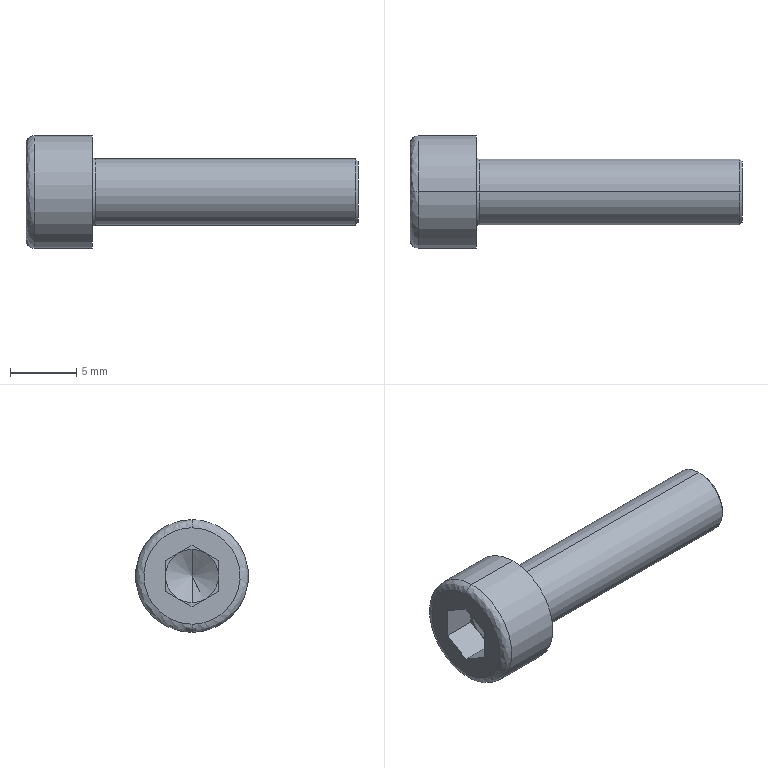Part | SolidWorks | features BaseBody 1 | 1 solid | 27 faces | box 25 x 8.5 x 8.5 mm | volume 634.624 mm3 | plane 15 | spline 4 | cylinder 4 | cone 4 | commonest cylinder face diameters 5 x2 8.5 x2
STEP:
#1=CARTESIAN_POINT('',(5.,0.,2.7));
#2=VERTEX_POINT('',#1);
#3=CARTESIAN_POINT('',(5.,0.,-2.7));
#4=VERTEX_POINT('',#3);
#5=CARTESIAN_POINT('',(5.,0.,2.7));
#6=CARTESIAN_POINT('',(5.,0.1716,2.7));
#7=CARTESIAN_POINT('',(5.,0.4245,2.676));
#8=CARTESIAN_POINT('',(5.,0.7118,2.607));
#9=CARTESIAN_POINT('',(5.,0.8535,2.562));
#10=CARTESIAN_POINT('',(5.,0.9138,2.541));
#11=CARTESIAN_POINT('',(5.,0.9539,2.526));
#12=CARTESIAN_POINT('',(5.,0.9722,2.519));
#13=CARTESIAN_POINT('',(5.,1.34,2.373));
#14=CARTESIAN_POINT('',(5.,1.646,2.172));
#15=CARTESIAN_POINT('',(5.,2.041,1.778));
#16=CARTESIAN_POINT('',(5.,2.215,1.564));
#17=CARTESIAN_POINT('',(5.,2.376,1.288));
#18=CARTESIAN_POINT('',(5.,2.447,1.143));
#19=CARTESIAN_POINT('',(5.,2.475,1.08));
#20=CARTESIAN_POINT('',(5.,2.493,1.037));
#21=CARTESIAN_POINT('',(5.,2.503,1.014));
#22=CARTESIAN_POINT('',(5.,2.637,0.675));
#23=CARTESIAN_POINT('',(5.,2.7,0.343));
#24=CARTESIAN_POINT('',(5.,2.7,-0.1715));
#25=CARTESIAN_POINT('',(5.,2.676,-0.4243));
#26=CARTESIAN_POINT('',(5.,2.607,-0.7117));
#27=CARTESIAN_POINT('',(5.,2.562,-0.8534));
#28=CARTESIAN_POINT('',(5.,2.541,-0.9137));
#29=CARTESIAN_POINT('',(5.,2.526,-0.9539));
#30=CARTESIAN_POINT('',(5.,2.519,-0.9722));
#31=CARTESIAN_POINT('',(5.,2.373,-1.34));
#32=CARTESIAN_POINT('',(5.,2.172,-1.646));
#33=CARTESIAN_POINT('',(5.,1.778,-2.041));
#34=CARTESIAN_POINT('',(5.,1.564,-2.215));
#35=CARTESIAN_POINT('',(5.,1.288,-2.376));
#36=CARTESIAN_POINT('',(5.,1.143,-2.447));
#37=CARTESIAN_POINT('',(5.,1.08,-2.475));
#38=CARTESIAN_POINT('',(5.,1.037,-2.493));
#39=CARTESIAN_POINT('',(5.,1.014,-2.503));
#40=CARTESIAN_POINT('',(5.,0.6748,-2.637));
#41=CARTESIAN_POINT('',(5.,0.3435,-2.7));
#42=CARTESIAN_POINT('',(5.,0.,-2.7));
#43=B_SPLINE_CURVE_WITH_KNOTS('',3,(#5,#6,#7,#8,#9,#10,#11,#12,#13,#14,#15,#16,#17,#18,#19,#20,#21,#22,#23,#24,#25,#26,#27,#28,#29,#30,#31,#32,#33,#34,#35,#36,#37,#38,#39,#40,#41,#42),.UNSPECIFIED.,.F.,.F.,(4,1,1,1,2,2,2,1,1,1,2,2,2,1,1,1,2,2,2,1,1,1,2,2,4),(0.,0.0625,0.09375,0.1094,0.1172,0.125,0.25,0.3125,0.3437,0.3594,0.3672,0.375,0.5,0.5625,0.5937,0.6094,0.6172,0.625,0.75,0.8125,0.8437,0.8594,0.8672,0.875,1.),.UNSPECIFIED.);
#44=EDGE_CURVE('',#2,#4,#43,.T.);
#45=ORIENTED_EDGE('',*,*,#44,.F.);
#46=CARTESIAN_POINT('',(5.2,0.,2.5));
#47=VERTEX_POINT('',#46);
#48=CARTESIAN_POINT('',(5.2,0.,2.7));
#49=DIRECTION('',(0.,-1.,0.));
#50=DIRECTION('',(0.,0.,1.));
#51=AXIS2_PLACEMENT_3D('',#48,#49,#50);
#52=CIRCLE('',#51,0.2);
#53=EDGE_CURVE('',#2,#47,#52,.T.);
#54=ORIENTED_EDGE('',*,*,#53,.T.);
#55=CARTESIAN_POINT('',(5.2,0.,-2.5));
#56=VERTEX_POINT('',#55);
#57=CARTESIAN_POINT('',(5.2,0.,0.));
#58=DIRECTION('',(1.,0.,0.));
#59=DIRECTION('',(0.,0.,1.));
#60=AXIS2_PLACEMENT_3D('',#57,#58,#59);
#61=CIRCLE('',#60,2.5);
#62=EDGE_CURVE('',#56,#47,#61,.T.);
#63=ORIENTED_EDGE('',*,*,#62,.F.);
#64=CARTESIAN_POINT('',(5.2,0.,-2.7));
#65=DIRECTION('',(0.,1.,0.));
#66=DIRECTION('',(0.,0.,-1.));
#67=AXIS2_PLACEMENT_3D('',#64,#65,#66);
#68=CIRCLE('',#67,0.2);
#69=EDGE_CURVE('',#4,#56,#68,.T.);
#70=ORIENTED_EDGE('',*,*,#69,.F.);
#71=EDGE_LOOP('',(#45,#54,#63,#70));
#72=FACE_OUTER_BOUND('',#71,.T.);
#73=CARTESIAN_POINT('',(5.,0.,-2.7));
#74=CARTESIAN_POINT('',(5.,5.4,-2.7));
#75=CARTESIAN_POINT('',(5.,5.4,2.7));
#76=CARTESIAN_POINT('',(5.,0.,2.7));
#77=CARTESIAN_POINT('',(5.,0.,-2.583));
#78=CARTESIAN_POINT('',(5.,5.166,-2.583));
#79=CARTESIAN_POINT('',(5.,5.166,2.583));
#80=CARTESIAN_POINT('',(5.,0.,2.583));
#81=CARTESIAN_POINT('',(5.083,0.,-2.5));
#82=CARTESIAN_POINT('',(5.083,5.,-2.5));
#83=CARTESIAN_POINT('',(5.083,5.,2.5));
#84=CARTESIAN_POINT('',(5.083,0.,2.5));
#85=CARTESIAN_POINT('',(5.2,0.,-2.5));
#86=CARTESIAN_POINT('',(5.2,5.,-2.5));
#87=CARTESIAN_POINT('',(5.2,5.,2.5));
#88=CARTESIAN_POINT('',(5.2,0.,2.5));
#89=(BOUNDED_SURFACE()B_SPLINE_SURFACE(3,3,((#73,#74,#75,#76),(#77,#78,#79,#80),(#81,#82,#83,#84),(#85,#86,#87,#88)),.UNSPECIFIED.,.F.,.F.,.T.)B_SPLINE_SURFACE_WITH_KNOTS((4,4),(4,4),(0.,1.),(0.,1.),.UNSPECIFIED.)GEOMETRIC_REPRESENTATION_ITEM()RATIONAL_B_SPLINE_SURFACE(((1.,0.3333,0.3333,1.),(0.8047,0.2682,0.2682,0.8047),(0.8047,0.2682,0.2682,0.8047),(1.,0.3333,0.3333,1.)))REPRESENTATION_ITEM('')SURFACE());
#90=ADVANCED_FACE('',(#72),#89,.F.);
#91=CARTESIAN_POINT('',(0.625,0.,4.25));
#92=VERTEX_POINT('',#91);
#93=CARTESIAN_POINT('',(0.625,0.,-4.25));
#94=VERTEX_POINT('',#93);
#95=CARTESIAN_POINT('',(0.625,0.,0.));
#96=DIRECTION('',(1.,0.,0.));
#97=DIRECTION('',(0.,0.,1.));
#98=AXIS2_PLACEMENT_3D('',#95,#96,#97);
#99=CIRCLE('',#98,4.25);
#100=EDGE_CURVE('',#92,#94,#99,.T.);
#101=ORIENTED_EDGE('',*,*,#100,.F.);
#102=CARTESIAN_POINT('',(0.,0.,3.625));
#103=VERTEX_POINT('',#102);
#104=CARTESIAN_POINT('',(0.625,0.,3.625));
#105=DIRECTION('',(0.,-1.,0.));
#106=DIRECTION('',(0.,0.,1.));
#107=AXIS2_PLACEMENT_3D('',#104,#105,#106);
#108=CIRCLE('',#107,0.625);
#109=EDGE_CURVE('',#92,#103,#108,.T.);
#110=ORIENTED_EDGE('',*,*,#109,.T.);
#111=CARTESIAN_POINT('',(0.,0.,-3.625));
#112=VERTEX_POINT('',#111);
#113=CARTESIAN_POINT('',(0.,0.,3.625));
#114=CARTESIAN_POINT('',(0.,-7.25,3.625));
#115=CARTESIAN_POINT('',(0.,-7.25,-3.625));
#116=CARTESIAN_POINT('',(0.,0.,-3.625));
#117=(BOUNDED_CURVE()B_SPLINE_CURVE(3,(#113,#114,#115,#116),.UNSPECIFIED.,.F.,.F.)B_SPLINE_CURVE_WITH_KNOTS((4,4),(0.,1.),.UNSPECIFIED.)CURVE()GEOMETRIC_REPRESENTATION_ITEM()RATIONAL_B_SPLINE_CURVE((1.,0.3333,0.3333,1.))REPRESENTATION_ITEM(''));
#118=EDGE_CURVE('',#103,#112,#117,.T.);
#119=ORIENTED_EDGE('',*,*,#118,.T.);
#120=CARTESIAN_POINT('',(0.625,0.,-3.625));
#121=DIRECTION('',(0.,1.,0.));
#122=DIRECTION('',(0.,0.,-1.));
#123=AXIS2_PLACEMENT_3D('',#120,#121,#122);
#124=CIRCLE('',#123,0.625);
#125=EDGE_CURVE('',#94,#112,#124,.T.);
#126=ORIENTED_EDGE('',*,*,#125,.F.);
#127=EDGE_LOOP('',(#101,#110,#119,#126));
#128=FACE_OUTER_BOUND('',#127,.T.);
#129=CARTESIAN_POINT('',(0.625,0.,4.25));
#130=CARTESIAN_POINT('',(0.625,-8.5,4.25));
#131=CARTESIAN_POINT('',(0.625,-8.5,-4.25));
#132=CARTESIAN_POINT('',(0.625,0.,-4.25));
#133=CARTESIAN_POINT('',(0.2589,0.,4.25));
#134=CARTESIAN_POINT('',(0.2589,-8.5,4.25));
#135=CARTESIAN_POINT('',(0.2589,-8.5,-4.25));
#136=CARTESIAN_POINT('',(0.2589,0.,-4.25));
#137=CARTESIAN_POINT('',(0.,0.,3.991));
#138=CARTESIAN_POINT('',(0.,-7.982,3.991));
#139=CARTESIAN_POINT('',(0.,-7.982,-3.991));
#140=CARTESIAN_POINT('',(0.,0.,-3.991));
#141=CARTESIAN_POINT('',(0.,0.,3.625));
#142=CARTESIAN_POINT('',(0.,-7.25,3.625));
#143=CARTESIAN_POINT('',(0.,-7.25,-3.625));
#144=CARTESIAN_POINT('',(0.,0.,-3.625));
#145=(BOUNDED_SURFACE()B_SPLINE_SURFACE(3,3,((#129,#130,#131,#132),(#133,#134,#135,#136),(#137,#138,#139,#140),(#141,#142,#143,#144)),.UNSPECIFIED.,.F.,.F.,.T.)B_SPLINE_SURFACE_WITH_KNOTS((4,4),(4,4),(0.,1.),(0.,1.),.UNSPECIFIED.)GEOMETRIC_REPRESENTATION_ITEM()RATIONAL_B_SPLINE_SURFACE(((1.,0.3333,0.3333,1.),(0.8047,0.2682,0.2682,0.8047),(0.8047,0.2682,0.2682,0.8047),(1.,0.3333,0.3333,1.)))REPRESENTATION_ITEM('')SURFACE());
#146=ADVANCED_FACE('',(#128),#145,.T.);
#147=CARTESIAN_POINT('',(24.8,0.,2.5));
#148=VERTEX_POINT('',#147);
#149=CARTESIAN_POINT('',(24.8,0.,-2.5));
#150=VERTEX_POINT('',#149);
#151=CARTESIAN_POINT('',(24.8,0.,0.));
#152=DIRECTION('',(-1.,0.,0.));
#153=DIRECTION('',(0.,0.,1.));
#154=AXIS2_PLACEMENT_3D('',#151,#152,#153);
#155=CIRCLE('',#154,2.5);
#156=EDGE_CURVE('',#148,#150,#155,.T.);
#157=ORIENTED_EDGE('',*,*,#156,.T.);
#158=CARTESIAN_POINT('',(25.,0.,-2.5));
#159=DIRECTION('',(-1.,0.,0.));
#160=VECTOR('',#159,1000.);
#161=LINE('',#158,#160);
#162=EDGE_CURVE('',#150,#56,#161,.T.);
#163=ORIENTED_EDGE('',*,*,#162,.T.);
#164=ORIENTED_EDGE('',*,*,#62,.T.);
#165=CARTESIAN_POINT('',(25.,0.,2.5));
#166=DIRECTION('',(-1.,0.,0.));
#167=VECTOR('',#166,1000.);
#168=LINE('',#165,#167);
#169=EDGE_CURVE('',#148,#47,#168,.T.);
#170=ORIENTED_EDGE('',*,*,#169,.F.);
#171=EDGE_LOOP('',(#157,#163,#164,#170));
#172=FACE_OUTER_BOUND('',#171,.T.);
#173=CARTESIAN_POINT('',(25.,0.,0.));
#174=DIRECTION('',(-1.,0.,0.));
#175=DIRECTION('',(0.,0.,1.));
#176=AXIS2_PLACEMENT_3D('',#173,#174,#175);
#177=CYLINDRICAL_SURFACE('',#176,2.5);
#178=ADVANCED_FACE('',(#172),#177,.T.);
#179=CARTESIAN_POINT('',(25.,0.,2.3));
#180=VERTEX_POINT('',#179);
#181=CARTESIAN_POINT('',(25.,0.,-2.3));
#182=VERTEX_POINT('',#181);
#183=CARTESIAN_POINT('',(25.,0.,0.));
#184=DIRECTION('',(-1.,0.,0.));
#185=DIRECTION('',(0.,0.,1.));
#186=AXIS2_PLACEMENT_3D('',#183,#184,#185);
#187=CIRCLE('',#186,2.3);
#188=EDGE_CURVE('',#180,#182,#187,.T.);
#189=ORIENTED_EDGE('',*,*,#188,.T.);
#190=CARTESIAN_POINT('',(24.8,0.,-2.5));
#191=DIRECTION('',(-0.7071,0.,-0.7071));
#192=VECTOR('',#191,1000.);
#193=LINE('',#190,#192);
#194=EDGE_CURVE('',#182,#150,#193,.T.);
#195=ORIENTED_EDGE('',*,*,#194,.T.);
#196=ORIENTED_EDGE('',*,*,#156,.F.);
#197=CARTESIAN_POINT('',(24.8,0.,2.5));
#198=DIRECTION('',(-0.7071,0.,0.7071));
#199=VECTOR('',#198,1000.);
#200=LINE('',#197,#199);
#201=EDGE_CURVE('',#180,#148,#200,.T.);
#202=ORIENTED_EDGE('',*,*,#201,.F.);
#203=EDGE_LOOP('',(#189,#195,#196,#202));
#204=FACE_OUTER_BOUND('',#203,.T.);
#205=CARTESIAN_POINT('',(24.8,0.,0.));
#206=DIRECTION('',(-1.,0.,0.));
#207=DIRECTION('',(0.,0.,1.));
#208=AXIS2_PLACEMENT_3D('',#205,#206,#207);
#209=CONICAL_SURFACE('',#208,2.5,0.7854);
#210=ADVANCED_FACE('',(#204),#209,.T.);
#211=CARTESIAN_POINT('',(5.,0.,-4.25));
#212=VERTEX_POINT('',#211);
#213=CARTESIAN_POINT('',(5.,0.,4.25));
#214=VERTEX_POINT('',#213);
#215=CARTESIAN_POINT('',(5.,0.,0.));
#216=DIRECTION('',(1.,0.,0.));
#217=DIRECTION('',(0.,0.,1.));
#218=AXIS2_PLACEMENT_3D('',#215,#216,#217);
#219=CIRCLE('',#218,4.25);
#220=EDGE_CURVE('',#212,#214,#219,.T.);
#221=ORIENTED_EDGE('',*,*,#220,.F.);
#222=CARTESIAN_POINT('',(5.,0.,-4.25));
#223=DIRECTION('',(-1.,0.,0.));
#224=VECTOR('',#223,1000.);
#225=LINE('',#222,#224);
#226=EDGE_CURVE('',#212,#94,#225,.T.);
#227=ORIENTED_EDGE('',*,*,#226,.T.);
#228=CARTESIAN_POINT('',(0.625,0.,0.));
#229=DIRECTION('',(1.,0.,0.));
#230=DIRECTION('',(0.,0.,1.));
#231=AXIS2_PLACEMENT_3D('',#228,#229,#230);
#232=CIRCLE('',#231,4.25);
#233=EDGE_CURVE('',#94,#92,#232,.T.);
#234=ORIENTED_EDGE('',*,*,#233,.T.);
#235=CARTESIAN_POINT('',(5.,0.,4.25));
#236=DIRECTION('',(-1.,0.,0.));
#237=VECTOR('',#236,1000.);
#238=LINE('',#235,#237);
#239=EDGE_CURVE('',#214,#92,#238,.T.);
#240=ORIENTED_EDGE('',*,*,#239,.F.);
#241=EDGE_LOOP('',(#221,#227,#234,#240));
#242=FACE_OUTER_BOUND('',#241,.T.);
#243=CARTESIAN_POINT('',(5.,0.,0.));
#244=DIRECTION('',(-1.,0.,0.));
#245=DIRECTION('',(0.,0.,1.));
#246=AXIS2_PLACEMENT_3D('',#243,#244,#245);
#247=CYLINDRICAL_SURFACE('',#246,4.25);
#248=ADVANCED_FACE('',(#242),#247,.T.);
#249=CARTESIAN_POINT('',(3.655,0.,0.));
#250=VERTEX_POINT('',#249);
#251=CARTESIAN_POINT('',(2.5,0.,2.));
#252=VERTEX_POINT('',#251);
#253=CARTESIAN_POINT('',(2.5,0.,2.));
#254=DIRECTION('',(-0.5,0.,0.866));
#255=VECTOR('',#254,1000.);
#256=LINE('',#253,#255);
#257=EDGE_CURVE('',#250,#252,#256,.T.);
#258=ORIENTED_EDGE('',*,*,#257,.F.);
#259=CARTESIAN_POINT('',(2.5,0.,-2.));
#260=VERTEX_POINT('',#259);
#261=CARTESIAN_POINT('',(2.5,0.,-2.));
#262=DIRECTION('',(-0.5,0.,-0.866));
#263=VECTOR('',#262,1000.);
#264=LINE('',#261,#263);
#265=EDGE_CURVE('',#250,#260,#264,.T.);
#266=ORIENTED_EDGE('',*,*,#265,.T.);
#267=CARTESIAN_POINT('',(2.5,-1.,-1.732));
#268=VERTEX_POINT('',#267);
#269=CARTESIAN_POINT('',(2.5,0.,0.));
#270=DIRECTION('',(1.,0.,0.));
#271=DIRECTION('',(0.,0.,1.));
#272=AXIS2_PLACEMENT_3D('',#269,#270,#271);
#273=CIRCLE('',#272,2.);
#274=EDGE_CURVE('',#268,#260,#273,.T.);
#275=ORIENTED_EDGE('',*,*,#274,.F.);
#276=CARTESIAN_POINT('',(2.5,-2.,0.));
#277=VERTEX_POINT('',#276);
#278=CARTESIAN_POINT('',(2.5,0.,0.));
#279=DIRECTION('',(-1.,0.,0.));
#280=DIRECTION('',(0.,0.,1.));
#281=AXIS2_PLACEMENT_3D('',#278,#279,#280);
#282=CIRCLE('',#281,2.);
#283=EDGE_CURVE('',#268,#277,#282,.T.);
#284=ORIENTED_EDGE('',*,*,#283,.T.);
#285=CARTESIAN_POINT('',(2.5,-1.,1.732));
#286=VERTEX_POINT('',#285);
#287=CARTESIAN_POINT('',(2.5,0.,0.));
#288=DIRECTION('',(1.,0.,0.));
#289=DIRECTION('',(0.,0.,1.));
#290=AXIS2_PLACEMENT_3D('',#287,#288,#289);
#291=CIRCLE('',#290,2.);
#292=EDGE_CURVE('',#286,#277,#291,.T.);
#293=ORIENTED_EDGE('',*,*,#292,.F.);
#294=CARTESIAN_POINT('',(2.5,0.,0.));
#295=DIRECTION('',(1.,0.,0.));
#296=DIRECTION('',(0.,0.,1.));
#297=AXIS2_PLACEMENT_3D('',#294,#295,#296);
#298=CIRCLE('',#297,2.);
#299=EDGE_CURVE('',#252,#286,#298,.T.);
#300=ORIENTED_EDGE('',*,*,#299,.F.);
#301=EDGE_LOOP('',(#258,#266,#275,#284,#293,#300));
#302=FACE_OUTER_BOUND('',#301,.T.);
#303=CARTESIAN_POINT('',(2.5,0.,0.));
#304=DIRECTION('',(-1.,0.,0.));
#305=DIRECTION('',(0.,0.,1.));
#306=AXIS2_PLACEMENT_3D('',#303,#304,#305);
#307=CONICAL_SURFACE('',#306,2.,1.047);
#308=ADVANCED_FACE('',(#302),#307,.F.);
#309=ORIENTED_EDGE('',*,*,#162,.F.);
#310=CARTESIAN_POINT('',(24.8,0.,0.));
#311=DIRECTION('',(-1.,0.,0.));
#312=DIRECTION('',(0.,0.,1.));
#313=AXIS2_PLACEMENT_3D('',#310,#311,#312);
#314=CIRCLE('',#313,2.5);
#315=EDGE_CURVE('',#150,#148,#314,.T.);
#316=ORIENTED_EDGE('',*,*,#315,.T.);
#317=ORIENTED_EDGE('',*,*,#169,.T.);
#318=CARTESIAN_POINT('',(5.2,0.,0.));
#319=DIRECTION('',(1.,0.,0.));
#320=DIRECTION('',(0.,0.,1.));
#321=AXIS2_PLACEMENT_3D('',#318,#319,#320);
#322=CIRCLE('',#321,2.5);
#323=EDGE_CURVE('',#47,#56,#322,.T.);
#324=ORIENTED_EDGE('',*,*,#323,.T.);
#325=EDGE_LOOP('',(#309,#316,#317,#324));
#326=FACE_OUTER_BOUND('',#325,.T.);
#327=CARTESIAN_POINT('',(25.,0.,0.));
#328=DIRECTION('',(-1.,0.,0.));
#329=DIRECTION('',(0.,0.,1.));
#330=AXIS2_PLACEMENT_3D('',#327,#328,#329);
#331=CYLINDRICAL_SURFACE('',#330,2.5);
#332=ADVANCED_FACE('',(#326),#331,.T.);
#333=ORIENTED_EDGE('',*,*,#53,.F.);
#334=CARTESIAN_POINT('',(5.,0.,-2.7));
#335=CARTESIAN_POINT('',(5.,-0.1716,-2.7));
#336=CARTESIAN_POINT('',(5.,-0.4245,-2.676));
#337=CARTESIAN_POINT('',(5.,-0.7118,-2.607));
#338=CARTESIAN_POINT('',(5.,-0.8535,-2.562));
#339=CARTESIAN_POINT('',(5.,-0.9138,-2.541));
#340=CARTESIAN_POINT('',(5.,-0.9539,-2.526));
#341=CARTESIAN_POINT('',(5.,-0.9722,-2.519));
#342=CARTESIAN_POINT('',(5.,-1.34,-2.373));
#343=CARTESIAN_POINT('',(5.,-1.646,-2.172));
#344=CARTESIAN_POINT('',(5.,-2.041,-1.778));
#345=CARTESIAN_POINT('',(5.,-2.215,-1.564));
#346=CARTESIAN_POINT('',(5.,-2.376,-1.288));
#347=CARTESIAN_POINT('',(5.,-2.447,-1.143));
#348=CARTESIAN_POINT('',(5.,-2.475,-1.08));
#349=CARTESIAN_POINT('',(5.,-2.493,-1.037));
#350=CARTESIAN_POINT('',(5.,-2.503,-1.014));
#351=CARTESIAN_POINT('',(5.,-2.637,-0.675));
#352=CARTESIAN_POINT('',(5.,-2.7,-0.343));
#353=CARTESIAN_POINT('',(5.,-2.7,0.1715));
#354=CARTESIAN_POINT('',(5.,-2.676,0.4243));
#355=CARTESIAN_POINT('',(5.,-2.607,0.7117));
#356=CARTESIAN_POINT('',(5.,-2.562,0.8534));
#357=CARTESIAN_POINT('',(5.,-2.541,0.9137));
#358=CARTESIAN_POINT('',(5.,-2.526,0.9539));
#359=CARTESIAN_POINT('',(5.,-2.519,0.9722));
#360=CARTESIAN_POINT('',(5.,-2.373,1.34));
#361=CARTESIAN_POINT('',(5.,-2.172,1.646));
#362=CARTESIAN_POINT('',(5.,-1.778,2.041));
#363=CARTESIAN_POINT('',(5.,-1.564,2.215));
#364=CARTESIAN_POINT('',(5.,-1.288,2.376));
#365=CARTESIAN_POINT('',(5.,-1.143,2.447));
#366=CARTESIAN_POINT('',(5.,-1.08,2.475));
#367=CARTESIAN_POINT('',(5.,-1.037,2.493));
#368=CARTESIAN_POINT('',(5.,-1.014,2.503));
#369=CARTESIAN_POINT('',(5.,-0.6748,2.637));
#370=CARTESIAN_POINT('',(5.,-0.3435,2.7));
#371=CARTESIAN_POINT('',(5.,0.,2.7));
#372=B_SPLINE_CURVE_WITH_KNOTS('',3,(#334,#335,#336,#337,#338,#339,#340,#341,#342,#343,#344,#345,#346,#347,#348,#349,#350,#351,#352,#353,#354,#355,#356,#357,#358,#359,#360,#361,#362,#363,#364,#365,#366,#367,#368,#369,#370,#371),.UNSPECIFIED.,.F.,.F.,(4,1,1,1,2,2,2,1,1,1,2,2,2,1,1,1,2,2,2,1,1,1,2,2,4),(0.,0.0625,0.09375,0.1094,0.1172,0.125,0.25,0.3125,0.3437,0.3594,0.3672,0.375,0.5,0.5625,0.5937,0.6094,0.6172,0.625,0.75,0.8125,0.8437,0.8594,0.8672,0.875,1.),.UNSPECIFIED.);
#373=EDGE_CURVE('',#4,#2,#372,.T.);
#374=ORIENTED_EDGE('',*,*,#373,.F.);
#375=ORIENTED_EDGE('',*,*,#69,.T.);
#376=ORIENTED_EDGE('',*,*,#323,.F.);
#377=EDGE_LOOP('',(#333,#374,#375,#376));
#378=FACE_OUTER_BOUND('',#377,.T.);
#379=CARTESIAN_POINT('',(5.,0.,2.7));
#380=CARTESIAN_POINT('',(5.,-5.4,2.7));
#381=CARTESIAN_POINT('',(5.,-5.4,-2.7));
#382=CARTESIAN_POINT('',(5.,0.,-2.7));
#383=CARTESIAN_POINT('',(5.,0.,2.583));
#384=CARTESIAN_POINT('',(5.,-5.166,2.583));
#385=CARTESIAN_POINT('',(5.,-5.166,-2.583));
#386=CARTESIAN_POINT('',(5.,0.,-2.583));
#387=CARTESIAN_POINT('',(5.083,0.,2.5));
#388=CARTESIAN_POINT('',(5.083,-5.,2.5));
#389=CARTESIAN_POINT('',(5.083,-5.,-2.5));
#390=CARTESIAN_POINT('',(5.083,0.,-2.5));
#391=CARTESIAN_POINT('',(5.2,0.,2.5));
#392=CARTESIAN_POINT('',(5.2,-5.,2.5));
#393=CARTESIAN_POINT('',(5.2,-5.,-2.5));
#394=CARTESIAN_POINT('',(5.2,0.,-2.5));
#395=(BOUNDED_SURFACE()B_SPLINE_SURFACE(3,3,((#379,#380,#381,#382),(#383,#384,#385,#386),(#387,#388,#389,#390),(#391,#392,#393,#394)),.UNSPECIFIED.,.F.,.F.,.T.)B_SPLINE_SURFACE_WITH_KNOTS((4,4),(4,4),(0.,1.),(0.,1.),.UNSPECIFIED.)GEOMETRIC_REPRESENTATION_ITEM()RATIONAL_B_SPLINE_SURFACE(((1.,0.3333,0.3333,1.),(0.8047,0.2682,0.2682,0.8047),(0.8047,0.2682,0.2682,0.8047),(1.,0.3333,0.3333,1.)))REPRESENTATION_ITEM('')SURFACE());
#396=ADVANCED_FACE('',(#378),#395,.F.);
#397=ORIENTED_EDGE('',*,*,#194,.F.);
#398=CARTESIAN_POINT('',(25.,0.,0.));
#399=DIRECTION('',(-1.,0.,0.));
#400=DIRECTION('',(0.,0.,1.));
#401=AXIS2_PLACEMENT_3D('',#398,#399,#400);
#402=CIRCLE('',#401,2.3);
#403=EDGE_CURVE('',#182,#180,#402,.T.);
#404=ORIENTED_EDGE('',*,*,#403,.T.);
#405=ORIENTED_EDGE('',*,*,#201,.T.);
#406=ORIENTED_EDGE('',*,*,#315,.F.);
#407=EDGE_LOOP('',(#397,#404,#405,#406));
#408=FACE_OUTER_BOUND('',#407,.T.);
#409=CARTESIAN_POINT('',(24.8,0.,0.));
#410=DIRECTION('',(-1.,0.,0.));
#411=DIRECTION('',(0.,0.,1.));
#412=AXIS2_PLACEMENT_3D('',#409,#410,#411);
#413=CONICAL_SURFACE('',#412,2.5,0.7854);
#414=ADVANCED_FACE('',(#408),#413,.T.);
#415=CARTESIAN_POINT('',(5.,0.,0.));
#416=DIRECTION('',(1.,0.,0.));
#417=DIRECTION('',(0.,0.,1.));
#418=AXIS2_PLACEMENT_3D('',#415,#416,#417);
#419=CIRCLE('',#418,4.25);
#420=EDGE_CURVE('',#214,#212,#419,.T.);
#421=ORIENTED_EDGE('',*,*,#420,.T.);
#422=ORIENTED_EDGE('',*,*,#220,.T.);
#423=EDGE_LOOP('',(#421,#422));
#424=FACE_OUTER_BOUND('',#423,.T.);
#425=ORIENTED_EDGE('',*,*,#373,.T.);
#426=ORIENTED_EDGE('',*,*,#44,.T.);
#427=EDGE_LOOP('',(#425,#426));
#428=FACE_BOUND('',#427,.T.);
#429=CARTESIAN_POINT('',(5.,0.,0.));
#430=DIRECTION('',(1.,0.,0.));
#431=DIRECTION('',(0.,0.,-1.));
#432=AXIS2_PLACEMENT_3D('',#429,#430,#431);
#433=PLANE('',#432);
#434=ADVANCED_FACE('',(#424,#428),#433,.T.);
#435=ORIENTED_EDGE('',*,*,#188,.F.);
#436=ORIENTED_EDGE('',*,*,#403,.F.);
#437=EDGE_LOOP('',(#435,#436));
#438=FACE_OUTER_BOUND('',#437,.T.);
#439=CARTESIAN_POINT('',(25.,0.,0.));
#440=DIRECTION('',(1.,0.,0.));
#441=DIRECTION('',(0.,0.,-1.));
#442=AXIS2_PLACEMENT_3D('',#439,#440,#441);
#443=PLANE('',#442);
#444=ADVANCED_FACE('',(#438),#443,.T.);
#445=ORIENTED_EDGE('',*,*,#226,.F.);
#446=ORIENTED_EDGE('',*,*,#420,.F.);
#447=ORIENTED_EDGE('',*,*,#239,.T.);
#448=ORIENTED_EDGE('',*,*,#100,.T.);
#449=EDGE_LOOP('',(#445,#446,#447,#448));
#450=FACE_OUTER_BOUND('',#449,.T.);
#451=CARTESIAN_POINT('',(5.,0.,0.));
#452=DIRECTION('',(-1.,0.,0.));
#453=DIRECTION('',(0.,0.,1.));
#454=AXIS2_PLACEMENT_3D('',#451,#452,#453);
#455=CYLINDRICAL_SURFACE('',#454,4.25);
#456=ADVANCED_FACE('',(#450),#455,.T.);
#457=ORIENTED_EDGE('',*,*,#109,.F.);
#458=ORIENTED_EDGE('',*,*,#233,.F.);
#459=ORIENTED_EDGE('',*,*,#125,.T.);
#460=CARTESIAN_POINT('',(0.,0.,-3.625));
#461=CARTESIAN_POINT('',(0.,7.25,-3.625));
#462=CARTESIAN_POINT('',(0.,7.25,3.625));
#463=CARTESIAN_POINT('',(0.,0.,3.625));
#464=(BOUNDED_CURVE()B_SPLINE_CURVE(3,(#460,#461,#462,#463),.UNSPECIFIED.,.F.,.F.)B_SPLINE_CURVE_WITH_KNOTS((4,4),(0.,1.),.UNSPECIFIED.)CURVE()GEOMETRIC_REPRESENTATION_ITEM()RATIONAL_B_SPLINE_CURVE((1.,0.3333,0.3333,1.))REPRESENTATION_ITEM(''));
#465=EDGE_CURVE('',#112,#103,#464,.T.);
#466=ORIENTED_EDGE('',*,*,#465,.T.);
#467=EDGE_LOOP('',(#457,#458,#459,#466));
#468=FACE_OUTER_BOUND('',#467,.T.);
#469=CARTESIAN_POINT('',(0.625,0.,-4.25));
#470=CARTESIAN_POINT('',(0.625,8.5,-4.25));
#471=CARTESIAN_POINT('',(0.625,8.5,4.25));
#472=CARTESIAN_POINT('',(0.625,0.,4.25));
#473=CARTESIAN_POINT('',(0.2589,0.,-4.25));
#474=CARTESIAN_POINT('',(0.2589,8.5,-4.25));
#475=CARTESIAN_POINT('',(0.2589,8.5,4.25));
#476=CARTESIAN_POINT('',(0.2589,0.,4.25));
#477=CARTESIAN_POINT('',(0.,0.,-3.991));
#478=CARTESIAN_POINT('',(0.,7.982,-3.991));
#479=CARTESIAN_POINT('',(0.,7.982,3.991));
#480=CARTESIAN_POINT('',(0.,0.,3.991));
#481=CARTESIAN_POINT('',(0.,0.,-3.625));
#482=CARTESIAN_POINT('',(0.,7.25,-3.625));
#483=CARTESIAN_POINT('',(0.,7.25,3.625));
#484=CARTESIAN_POINT('',(0.,0.,3.625));
#485=(BOUNDED_SURFACE()B_SPLINE_SURFACE(3,3,((#469,#470,#471,#472),(#473,#474,#475,#476),(#477,#478,#479,#480),(#481,#482,#483,#484)),.UNSPECIFIED.,.F.,.F.,.T.)B_SPLINE_SURFACE_WITH_KNOTS((4,4),(4,4),(0.,1.),(0.,1.),.UNSPECIFIED.)GEOMETRIC_REPRESENTATION_ITEM()RATIONAL_B_SPLINE_SURFACE(((1.,0.3333,0.3333,1.),(0.8047,0.2682,0.2682,0.8047),(0.8047,0.2682,0.2682,0.8047),(1.,0.3333,0.3333,1.)))REPRESENTATION_ITEM('')SURFACE());
#486=ADVANCED_FACE('',(#468),#485,.T.);
#487=CARTESIAN_POINT('',(0.,2.,1.155));
#488=VERTEX_POINT('',#487);
#489=CARTESIAN_POINT('',(0.,2.,-1.155));
#490=VERTEX_POINT('',#489);
#491=CARTESIAN_POINT('',(0.,2.,0.));
#492=DIRECTION('',(0.,0.,-1.));
#493=VECTOR('',#492,1000.);
#494=LINE('',#491,#493);
#495=EDGE_CURVE('',#488,#490,#494,.T.);
#496=ORIENTED_EDGE('',*,*,#495,.F.);
#497=CARTESIAN_POINT('',(0.,0.,2.309));
#498=VERTEX_POINT('',#497);
#499=CARTESIAN_POINT('',(0.,0.,2.309));
#500=DIRECTION('',(0.,0.866,-0.5));
#501=VECTOR('',#500,1000.);
#502=LINE('',#499,#501);
#503=EDGE_CURVE('',#498,#488,#502,.T.);
#504=ORIENTED_EDGE('',*,*,#503,.F.);
#505=CARTESIAN_POINT('',(0.,-2.,1.155));
#506=VERTEX_POINT('',#505);
#507=CARTESIAN_POINT('',(0.,-2.,1.155));
#508=DIRECTION('',(0.,0.866,0.5));
#509=VECTOR('',#508,1000.);
#510=LINE('',#507,#509);
#511=EDGE_CURVE('',#506,#498,#510,.T.);
#512=ORIENTED_EDGE('',*,*,#511,.F.);
#513=CARTESIAN_POINT('',(0.,-2.,-1.155));
#514=VERTEX_POINT('',#513);
#515=CARTESIAN_POINT('',(0.,-2.,0.));
#516=DIRECTION('',(0.,0.,1.));
#517=VECTOR('',#516,1000.);
#518=LINE('',#515,#517);
#519=EDGE_CURVE('',#514,#506,#518,.T.);
#520=ORIENTED_EDGE('',*,*,#519,.F.);
#521=CARTESIAN_POINT('',(0.,0.,-2.309));
#522=VERTEX_POINT('',#521);
#523=CARTESIAN_POINT('',(0.,0.,-2.309));
#524=DIRECTION('',(0.,-0.866,0.5));
#525=VECTOR('',#524,1000.);
#526=LINE('',#523,#525);
#527=EDGE_CURVE('',#522,#514,#526,.T.);
#528=ORIENTED_EDGE('',*,*,#527,.F.);
#529=CARTESIAN_POINT('',(0.,2.,-1.155));
#530=DIRECTION('',(0.,-0.866,-0.5));
#531=VECTOR('',#530,1000.);
#532=LINE('',#529,#531);
#533=EDGE_CURVE('',#490,#522,#532,.T.);
#534=ORIENTED_EDGE('',*,*,#533,.F.);
#535=EDGE_LOOP('',(#496,#504,#512,#520,#528,#534));
#536=FACE_BOUND('',#535,.T.);
#537=ORIENTED_EDGE('',*,*,#465,.F.);
#538=ORIENTED_EDGE('',*,*,#118,.F.);
#539=EDGE_LOOP('',(#537,#538));
#540=FACE_OUTER_BOUND('',#539,.T.);
#541=CARTESIAN_POINT('',(0.,0.,0.));
#542=DIRECTION('',(1.,0.,0.));
#543=DIRECTION('',(0.,0.,-1.));
#544=AXIS2_PLACEMENT_3D('',#541,#542,#543);
#545=PLANE('',#544);
#546=ADVANCED_FACE('',(#536,#540),#545,.F.);
#547=CARTESIAN_POINT('',(2.5,0.,-2.309));
#548=VERTEX_POINT('',#547);
#549=CARTESIAN_POINT('',(2.5,0.,-2.309));
#550=DIRECTION('',(1.,0.,0.));
#551=VECTOR('',#550,1000.);
#552=LINE('',#549,#551);
#553=EDGE_CURVE('',#522,#548,#552,.T.);
#554=ORIENTED_EDGE('',*,*,#553,.T.);
#555=CARTESIAN_POINT('',(2.5,1.,-1.732));
#556=VERTEX_POINT('',#555);
#557=CARTESIAN_POINT('',(2.5,0.,-2.309));
#558=DIRECTION('',(0.,0.866,0.5));
#559=VECTOR('',#558,1000.);
#560=LINE('',#557,#559);
#561=EDGE_CURVE('',#548,#556,#560,.T.);
#562=ORIENTED_EDGE('',*,*,#561,.T.);
#563=CARTESIAN_POINT('',(2.5,2.,-1.155));
#564=VERTEX_POINT('',#563);
#565=CARTESIAN_POINT('',(2.5,1.,-1.732));
#566=DIRECTION('',(0.,0.866,0.5));
#567=VECTOR('',#566,1000.);
#568=LINE('',#565,#567);
#569=EDGE_CURVE('',#556,#564,#568,.T.);
#570=ORIENTED_EDGE('',*,*,#569,.T.);
#571=CARTESIAN_POINT('',(2.5,2.,-1.155));
#572=DIRECTION('',(-1.,0.,0.));
#573=VECTOR('',#572,1000.);
#574=LINE('',#571,#573);
#575=EDGE_CURVE('',#564,#490,#574,.T.);
#576=ORIENTED_EDGE('',*,*,#575,.T.);
#577=ORIENTED_EDGE('',*,*,#533,.T.);
#578=EDGE_LOOP('',(#554,#562,#570,#576,#577));
#579=FACE_OUTER_BOUND('',#578,.T.);
#580=CARTESIAN_POINT('',(2.5,0.,-2.309));
#581=DIRECTION('',(0.,-0.5,0.866));
#582=DIRECTION('',(0.,-0.866,-0.5));
#583=AXIS2_PLACEMENT_3D('',#580,#581,#582);
#584=PLANE('',#583);
#585=ADVANCED_FACE('',(#579),#584,.T.);
#586=ORIENTED_EDGE('',*,*,#575,.F.);
#587=CARTESIAN_POINT('',(2.5,2.,0.));
#588=VERTEX_POINT('',#587);
#589=CARTESIAN_POINT('',(2.5,2.,-2.309));
#590=DIRECTION('',(0.,0.,1.));
#591=VECTOR('',#590,1000.);
#592=LINE('',#589,#591);
#593=EDGE_CURVE('',#564,#588,#592,.T.);
#594=ORIENTED_EDGE('',*,*,#593,.T.);
#595=CARTESIAN_POINT('',(2.5,2.,1.155));
#596=VERTEX_POINT('',#595);
#597=CARTESIAN_POINT('',(2.5,2.,-2.309));
#598=DIRECTION('',(0.,0.,1.));
#599=VECTOR('',#598,1000.);
#600=LINE('',#597,#599);
#601=EDGE_CURVE('',#588,#596,#600,.T.);
#602=ORIENTED_EDGE('',*,*,#601,.T.);
#603=CARTESIAN_POINT('',(2.5,2.,1.155));
#604=DIRECTION('',(-1.,0.,0.));
#605=VECTOR('',#604,1000.);
#606=LINE('',#603,#605);
#607=EDGE_CURVE('',#596,#488,#606,.T.);
#608=ORIENTED_EDGE('',*,*,#607,.T.);
#609=ORIENTED_EDGE('',*,*,#495,.T.);
#610=EDGE_LOOP('',(#586,#594,#602,#608,#609));
#611=FACE_OUTER_BOUND('',#610,.T.);
#612=CARTESIAN_POINT('',(2.5,2.,-1.155));
#613=DIRECTION('',(0.,-1.,0.));
#614=DIRECTION('',(0.,0.,-1.));
#615=AXIS2_PLACEMENT_3D('',#612,#613,#614);
#616=PLANE('',#615);
#617=ADVANCED_FACE('',(#611),#616,.T.);
#618=ORIENTED_EDGE('',*,*,#607,.F.);
#619=CARTESIAN_POINT('',(2.5,1.,1.732));
#620=VERTEX_POINT('',#619);
#621=CARTESIAN_POINT('',(2.5,2.,1.155));
#622=DIRECTION('',(0.,-0.866,0.5));
#623=VECTOR('',#622,1000.);
#624=LINE('',#621,#623);
#625=EDGE_CURVE('',#596,#620,#624,.T.);
#626=ORIENTED_EDGE('',*,*,#625,.T.);
#627=CARTESIAN_POINT('',(2.5,0.,2.309));
#628=VERTEX_POINT('',#627);
#629=CARTESIAN_POINT('',(2.5,2.,1.155));
#630=DIRECTION('',(0.,-0.866,0.5));
#631=VECTOR('',#630,1000.);
#632=LINE('',#629,#631);
#633=EDGE_CURVE('',#620,#628,#632,.T.);
#634=ORIENTED_EDGE('',*,*,#633,.T.);
#635=CARTESIAN_POINT('',(2.5,0.,2.309));
#636=DIRECTION('',(-1.,0.,0.));
#637=VECTOR('',#636,1000.);
#638=LINE('',#635,#637);
#639=EDGE_CURVE('',#628,#498,#638,.T.);
#640=ORIENTED_EDGE('',*,*,#639,.T.);
#641=ORIENTED_EDGE('',*,*,#503,.T.);
#642=EDGE_LOOP('',(#618,#626,#634,#640,#641));
#643=FACE_OUTER_BOUND('',#642,.T.);
#644=CARTESIAN_POINT('',(2.5,2.,1.155));
#645=DIRECTION('',(0.,-0.5,-0.866));
#646=DIRECTION('',(0.,0.866,-0.5));
#647=AXIS2_PLACEMENT_3D('',#644,#645,#646);
#648=PLANE('',#647);
#649=ADVANCED_FACE('',(#643),#648,.T.);
#650=ORIENTED_EDGE('',*,*,#639,.F.);
#651=CARTESIAN_POINT('',(2.5,0.,2.309));
#652=DIRECTION('',(0.,-0.866,-0.5));
#653=VECTOR('',#652,1000.);
#654=LINE('',#651,#653);
#655=EDGE_CURVE('',#628,#286,#654,.T.);
#656=ORIENTED_EDGE('',*,*,#655,.T.);
#657=CARTESIAN_POINT('',(2.5,-2.,1.155));
#658=VERTEX_POINT('',#657);
#659=CARTESIAN_POINT('',(2.5,-1.,1.732));
#660=DIRECTION('',(0.,-0.866,-0.5));
#661=VECTOR('',#660,1000.);
#662=LINE('',#659,#661);
#663=EDGE_CURVE('',#286,#658,#662,.T.);
#664=ORIENTED_EDGE('',*,*,#663,.T.);
#665=CARTESIAN_POINT('',(2.5,-2.,1.155));
#666=DIRECTION('',(-1.,0.,0.));
#667=VECTOR('',#666,1000.);
#668=LINE('',#665,#667);
#669=EDGE_CURVE('',#658,#506,#668,.T.);
#670=ORIENTED_EDGE('',*,*,#669,.T.);
#671=ORIENTED_EDGE('',*,*,#511,.T.);
#672=EDGE_LOOP('',(#650,#656,#664,#670,#671));
#673=FACE_OUTER_BOUND('',#672,.T.);
#674=CARTESIAN_POINT('',(2.5,0.,2.309));
#675=DIRECTION('',(0.,0.5,-0.866));
#676=DIRECTION('',(0.,0.866,0.5));
#677=AXIS2_PLACEMENT_3D('',#674,#675,#676);
#678=PLANE('',#677);
#679=ADVANCED_FACE('',(#673),#678,.T.);
#680=ORIENTED_EDGE('',*,*,#669,.F.);
#681=CARTESIAN_POINT('',(2.5,-2.,-2.309));
#682=DIRECTION('',(0.,0.,-1.));
#683=VECTOR('',#682,1000.);
#684=LINE('',#681,#683);
#685=EDGE_CURVE('',#658,#277,#684,.T.);
#686=ORIENTED_EDGE('',*,*,#685,.T.);
#687=CARTESIAN_POINT('',(2.5,-2.,-1.155));
#688=VERTEX_POINT('',#687);
#689=CARTESIAN_POINT('',(2.5,-2.,1.155));
#690=DIRECTION('',(0.,0.,-1.));
#691=VECTOR('',#690,1000.);
#692=LINE('',#689,#691);
#693=EDGE_CURVE('',#277,#688,#692,.T.);
#694=ORIENTED_EDGE('',*,*,#693,.T.);
#695=CARTESIAN_POINT('',(2.5,-2.,-1.155));
#696=DIRECTION('',(-1.,0.,0.));
#697=VECTOR('',#696,1000.);
#698=LINE('',#695,#697);
#699=EDGE_CURVE('',#688,#514,#698,.T.);
#700=ORIENTED_EDGE('',*,*,#699,.T.);
#701=ORIENTED_EDGE('',*,*,#519,.T.);
#702=EDGE_LOOP('',(#680,#686,#694,#700,#701));
#703=FACE_OUTER_BOUND('',#702,.T.);
#704=CARTESIAN_POINT('',(2.5,-2.,1.155));
#705=DIRECTION('',(0.,1.,0.));
#706=DIRECTION('',(0.,0.,1.));
#707=AXIS2_PLACEMENT_3D('',#704,#705,#706);
#708=PLANE('',#707);
#709=ADVANCED_FACE('',(#703),#708,.T.);
#710=ORIENTED_EDGE('',*,*,#699,.F.);
#711=CARTESIAN_POINT('',(2.5,-2.,-1.155));
#712=DIRECTION('',(0.,0.866,-0.5));
#713=VECTOR('',#712,1000.);
#714=LINE('',#711,#713);
#715=EDGE_CURVE('',#688,#268,#714,.T.);
#716=ORIENTED_EDGE('',*,*,#715,.T.);
#717=CARTESIAN_POINT('',(2.5,-2.,-1.155));
#718=DIRECTION('',(0.,0.866,-0.5));
#719=VECTOR('',#718,1000.);
#720=LINE('',#717,#719);
#721=EDGE_CURVE('',#268,#548,#720,.T.);
#722=ORIENTED_EDGE('',*,*,#721,.T.);
#723=ORIENTED_EDGE('',*,*,#553,.F.);
#724=ORIENTED_EDGE('',*,*,#527,.T.);
#725=EDGE_LOOP('',(#710,#716,#722,#723,#724));
#726=FACE_OUTER_BOUND('',#725,.T.);
#727=CARTESIAN_POINT('',(2.5,-2.,-1.155));
#728=DIRECTION('',(0.,0.5,0.866));
#729=DIRECTION('',(0.,-0.866,0.5));
#730=AXIS2_PLACEMENT_3D('',#727,#728,#729);
#731=PLANE('',#730);
#732=ADVANCED_FACE('',(#726),#731,.T.);
#733=ORIENTED_EDGE('',*,*,#274,.T.);
#734=CARTESIAN_POINT('',(2.5,0.,0.));
#735=DIRECTION('',(1.,0.,0.));
#736=DIRECTION('',(0.,0.,1.));
#737=AXIS2_PLACEMENT_3D('',#734,#735,#736);
#738=CIRCLE('',#737,2.);
#739=EDGE_CURVE('',#260,#556,#738,.T.);
#740=ORIENTED_EDGE('',*,*,#739,.T.);
#741=ORIENTED_EDGE('',*,*,#561,.F.);
#742=ORIENTED_EDGE('',*,*,#721,.F.);
#743=EDGE_LOOP('',(#733,#740,#741,#742));
#744=FACE_OUTER_BOUND('',#743,.T.);
#745=CARTESIAN_POINT('',(2.5,0.,-2.309));
#746=DIRECTION('',(1.,0.,0.));
#747=DIRECTION('',(0.,0.,-1.));
#748=AXIS2_PLACEMENT_3D('',#745,#746,#747);
#749=PLANE('',#748);
#750=ADVANCED_FACE('',(#744),#749,.F.);
#751=ORIENTED_EDGE('',*,*,#633,.F.);
#752=CARTESIAN_POINT('',(2.5,0.,0.));
#753=DIRECTION('',(1.,0.,0.));
#754=DIRECTION('',(0.,0.,1.));
#755=AXIS2_PLACEMENT_3D('',#752,#753,#754);
#756=CIRCLE('',#755,2.);
#757=EDGE_CURVE('',#620,#252,#756,.T.);
#758=ORIENTED_EDGE('',*,*,#757,.T.);
#759=ORIENTED_EDGE('',*,*,#299,.T.);
#760=ORIENTED_EDGE('',*,*,#655,.F.);
#761=EDGE_LOOP('',(#751,#758,#759,#760));
#762=FACE_OUTER_BOUND('',#761,.T.);
#763=CARTESIAN_POINT('',(2.5,0.,-2.309));
#764=DIRECTION('',(1.,0.,0.));
#765=DIRECTION('',(0.,0.,-1.));
#766=AXIS2_PLACEMENT_3D('',#763,#764,#765);
#767=PLANE('',#766);
#768=ADVANCED_FACE('',(#762),#767,.F.);
#769=ORIENTED_EDGE('',*,*,#715,.F.);
#770=ORIENTED_EDGE('',*,*,#693,.F.);
#771=ORIENTED_EDGE('',*,*,#283,.F.);
#772=EDGE_LOOP('',(#769,#770,#771));
#773=FACE_OUTER_BOUND('',#772,.T.);
#774=CARTESIAN_POINT('',(2.5,0.,-2.309));
#775=DIRECTION('',(1.,0.,0.));
#776=DIRECTION('',(0.,0.,-1.));
#777=AXIS2_PLACEMENT_3D('',#774,#775,#776);
#778=PLANE('',#777);
#779=ADVANCED_FACE('',(#773),#778,.F.);
#780=ORIENTED_EDGE('',*,*,#265,.F.);
#781=ORIENTED_EDGE('',*,*,#257,.T.);
#782=ORIENTED_EDGE('',*,*,#757,.F.);
#783=CARTESIAN_POINT('',(2.5,0.,0.));
#784=DIRECTION('',(1.,0.,0.));
#785=DIRECTION('',(0.,0.,1.));
#786=AXIS2_PLACEMENT_3D('',#783,#784,#785);
#787=CIRCLE('',#786,2.);
#788=EDGE_CURVE('',#588,#620,#787,.T.);
#789=ORIENTED_EDGE('',*,*,#788,.F.);
#790=CARTESIAN_POINT('',(2.5,0.,0.));
#791=DIRECTION('',(1.,0.,0.));
#792=DIRECTION('',(0.,0.,1.));
#793=AXIS2_PLACEMENT_3D('',#790,#791,#792);
#794=CIRCLE('',#793,2.);
#795=EDGE_CURVE('',#556,#588,#794,.T.);
#796=ORIENTED_EDGE('',*,*,#795,.F.);
#797=ORIENTED_EDGE('',*,*,#739,.F.);
#798=EDGE_LOOP('',(#780,#781,#782,#789,#796,#797));
#799=FACE_OUTER_BOUND('',#798,.T.);
#800=CARTESIAN_POINT('',(2.5,0.,0.));
#801=DIRECTION('',(-1.,0.,0.));
#802=DIRECTION('',(0.,0.,1.));
#803=AXIS2_PLACEMENT_3D('',#800,#801,#802);
#804=CONICAL_SURFACE('',#803,2.,1.047);
#805=ADVANCED_FACE('',(#799),#804,.F.);
#806=ORIENTED_EDGE('',*,*,#685,.F.);
#807=ORIENTED_EDGE('',*,*,#663,.F.);
#808=ORIENTED_EDGE('',*,*,#292,.T.);
#809=EDGE_LOOP('',(#806,#807,#808));
#810=FACE_OUTER_BOUND('',#809,.T.);
#811=CARTESIAN_POINT('',(2.5,0.,-2.309));
#812=DIRECTION('',(1.,0.,0.));
#813=DIRECTION('',(0.,0.,-1.));
#814=AXIS2_PLACEMENT_3D('',#811,#812,#813);
#815=PLANE('',#814);
#816=ADVANCED_FACE('',(#810),#815,.F.);
#817=ORIENTED_EDGE('',*,*,#625,.F.);
#818=ORIENTED_EDGE('',*,*,#601,.F.);
#819=ORIENTED_EDGE('',*,*,#788,.T.);
#820=EDGE_LOOP('',(#817,#818,#819));
#821=FACE_OUTER_BOUND('',#820,.T.);
#822=CARTESIAN_POINT('',(2.5,0.,-2.309));
#823=DIRECTION('',(1.,0.,0.));
#824=DIRECTION('',(0.,0.,-1.));
#825=AXIS2_PLACEMENT_3D('',#822,#823,#824);
#826=PLANE('',#825);
#827=ADVANCED_FACE('',(#821),#826,.F.);
#828=ORIENTED_EDGE('',*,*,#593,.F.);
#829=ORIENTED_EDGE('',*,*,#569,.F.);
#830=ORIENTED_EDGE('',*,*,#795,.T.);
#831=EDGE_LOOP('',(#828,#829,#830));
#832=FACE_OUTER_BOUND('',#831,.T.);
#833=CARTESIAN_POINT('',(2.5,0.,-2.309));
#834=DIRECTION('',(1.,0.,0.));
#835=DIRECTION('',(0.,0.,-1.));
#836=AXIS2_PLACEMENT_3D('',#833,#834,#835);
#837=PLANE('',#836);
#838=ADVANCED_FACE('',(#832),#837,.F.);
#839=CLOSED_SHELL('',(#90,#146,#178,#210,#248,#308,#332,#396,#414,#434,#444,#456,#486,#546,#585,#617,#649,#679,#709,#732,#750,#768,#779,#805,#816,#827,#838));
#840=MANIFOLD_SOLID_BREP('',#839);
#841=CARTESIAN_POINT('',(0.,0.,0.));
#842=DIRECTION('',(0.,0.,1.));
#843=DIRECTION('',(1.,0.,0.));
#844=AXIS2_PLACEMENT_3D('',#841,#842,#843);
#845=(LENGTH_UNIT()NAMED_UNIT(*)SI_UNIT(.MILLI.,.METRE.));
#846=UNCERTAINTY_MEASURE_WITH_UNIT(LENGTH_MEASURE(0.00001),#845,'','');
#847=(NAMED_UNIT(*)PLANE_ANGLE_UNIT()SI_UNIT($,.RADIAN.));
#848=(NAMED_UNIT(*)SI_UNIT($,.STERADIAN.)SOLID_ANGLE_UNIT());
#849=(GEOMETRIC_REPRESENTATION_CONTEXT(3)GLOBAL_UNCERTAINTY_ASSIGNED_CONTEXT((#846))GLOBAL_UNIT_ASSIGNED_CONTEXT((#845,#847,#848))REPRESENTATION_CONTEXT('',''));
#850=ADVANCED_BREP_SHAPE_REPRESENTATION('',(#840,#844),#849);